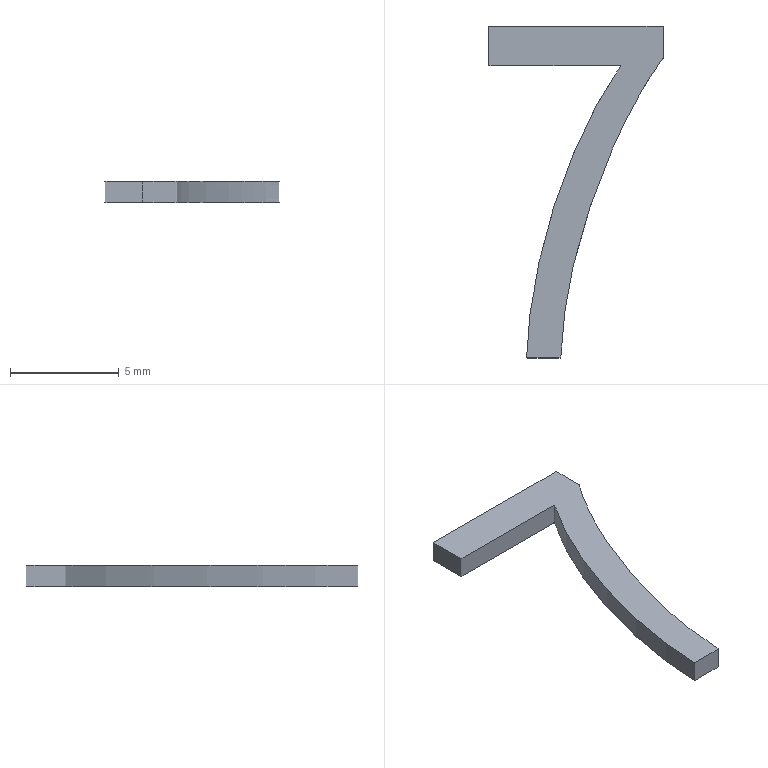Part | STEP file | lll_id1442_x_t | 1 solid | 3 faces | box 7.993 x 15.234 x 1 mm | volume 34.068 mm3 | plane 2 | other 1